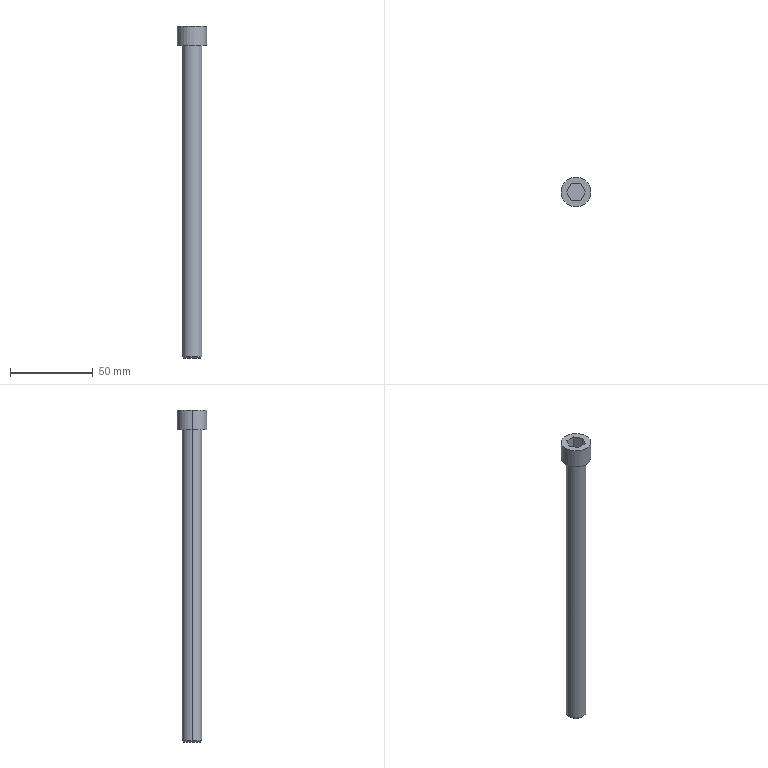Part | Creo | 1 solid | 16 faces | box 18 x 18 x 201 mm | volume 23734 mm3 | plane 10 | cylinder 4 | cone 2 | commonest cylinder face diameters 12 x2 18 x2
STEP:
#1=CARTESIAN_POINT('',(0.,0.,0.));
#2=DIRECTION('',(0.,0.,1.));
#3=DIRECTION('',(1.,0.,0.));
#4=AXIS2_PLACEMENT_3D('',#1,#2,#3);
#5=CARTESIAN_POINT('',(190.927,265.543,96.956));
#6=VERTEX_POINT('',#5);
#7=CARTESIAN_POINT('',(202.927,265.543,96.956));
#8=VERTEX_POINT('',#7);
#9=CARTESIAN_POINT('',(196.927,265.543,96.956));
#10=DIRECTION('',(0.,0.,-1.));
#11=DIRECTION('',(-1.,0.,0.));
#12=AXIS2_PLACEMENT_3D('',#9,#10,#11);
#13=CIRCLE('',#12,6.);
#14=EDGE_CURVE('',#6,#8,#13,.T.);
#15=ORIENTED_EDGE('',*,*,#14,.T.);
#16=CARTESIAN_POINT('',(202.927,265.543,285.245));
#17=VERTEX_POINT('',#16);
#18=CARTESIAN_POINT('',(202.927,265.543,285.245));
#19=DIRECTION('',(0.,0.,-1.));
#20=VECTOR('',#19,188.29);
#21=LINE('',#18,#20);
#22=EDGE_CURVE('',#17,#8,#21,.T.);
#23=ORIENTED_EDGE('',*,*,#22,.F.);
#24=CARTESIAN_POINT('',(190.927,265.543,285.245));
#25=VERTEX_POINT('',#24);
#26=CARTESIAN_POINT('',(196.927,265.543,285.245));
#27=DIRECTION('',(0.,0.,1.));
#28=DIRECTION('',(1.,0.,0.));
#29=AXIS2_PLACEMENT_3D('',#26,#27,#28);
#30=CIRCLE('',#29,6.);
#31=EDGE_CURVE('',#17,#25,#30,.T.);
#32=ORIENTED_EDGE('',*,*,#31,.T.);
#33=CARTESIAN_POINT('',(190.927,265.543,285.245));
#34=DIRECTION('',(0.,0.,-1.));
#35=VECTOR('',#34,188.29);
#36=LINE('',#33,#35);
#37=EDGE_CURVE('',#25,#6,#36,.T.);
#38=ORIENTED_EDGE('',*,*,#37,.T.);
#39=EDGE_LOOP('',(#15,#23,#32,#38));
#40=FACE_OUTER_BOUND('',#39,.F.);
#41=CARTESIAN_POINT('',(196.927,265.543,285.245));
#42=DIRECTION('',(0.,0.,-1.));
#43=DIRECTION('',(-1.,0.,0.));
#44=AXIS2_PLACEMENT_3D('',#41,#42,#43);
#45=CYLINDRICAL_SURFACE('',#44,6.);
#46=ADVANCED_FACE('',(#40),#45,.T.);
#47=CARTESIAN_POINT('',(191.637,265.543,96.245));
#48=VERTEX_POINT('',#47);
#49=CARTESIAN_POINT('',(202.216,265.543,96.245));
#50=VERTEX_POINT('',#49);
#51=CARTESIAN_POINT('',(196.927,265.543,96.245));
#52=DIRECTION('',(0.,0.,-1.));
#53=DIRECTION('',(-1.,0.,0.));
#54=AXIS2_PLACEMENT_3D('',#51,#52,#53);
#55=CIRCLE('',#54,5.29);
#56=EDGE_CURVE('',#48,#50,#55,.T.);
#57=ORIENTED_EDGE('',*,*,#56,.T.);
#58=CARTESIAN_POINT('',(202.216,265.543,96.245));
#59=DIRECTION('',(0.7071,0.,0.7071));
#60=VECTOR('',#59,1.005);
#61=LINE('',#58,#60);
#62=EDGE_CURVE('',#50,#8,#61,.T.);
#63=ORIENTED_EDGE('',*,*,#62,.T.);
#64=ORIENTED_EDGE('',*,*,#14,.F.);
#65=CARTESIAN_POINT('',(191.637,265.543,96.245));
#66=DIRECTION('',(-0.7071,0.,0.7071));
#67=VECTOR('',#66,1.005);
#68=LINE('',#65,#67);
#69=EDGE_CURVE('',#48,#6,#68,.T.);
#70=ORIENTED_EDGE('',*,*,#69,.F.);
#71=EDGE_LOOP('',(#57,#63,#64,#70));
#72=FACE_OUTER_BOUND('',#71,.F.);
#73=CARTESIAN_POINT('',(196.927,265.543,96.601));
#74=DIRECTION('',(0.,0.,1.));
#75=DIRECTION('',(1.,0.,0.));
#76=AXIS2_PLACEMENT_3D('',#73,#74,#75);
#77=CONICAL_SURFACE('',#76,5.645,45.);
#78=ADVANCED_FACE('',(#72),#77,.T.);
#79=CARTESIAN_POINT('',(196.927,265.543,96.245));
#80=DIRECTION('',(0.,0.,-1.));
#81=DIRECTION('',(1.,0.,0.));
#82=AXIS2_PLACEMENT_3D('',#79,#80,#81);
#83=CIRCLE('',#82,5.29);
#84=EDGE_CURVE('',#50,#48,#83,.T.);
#85=ORIENTED_EDGE('',*,*,#84,.F.);
#86=ORIENTED_EDGE('',*,*,#56,.F.);
#87=EDGE_LOOP('',(#85,#86));
#88=FACE_OUTER_BOUND('',#87,.F.);
#89=CARTESIAN_POINT('',(196.927,265.543,96.245));
#90=DIRECTION('',(0.,0.,1.));
#91=DIRECTION('',(1.,0.,0.));
#92=AXIS2_PLACEMENT_3D('',#89,#90,#91);
#93=PLANE('',#92);
#94=ADVANCED_FACE('',(#88),#93,.F.);
#95=ORIENTED_EDGE('',*,*,#84,.T.);
#96=ORIENTED_EDGE('',*,*,#69,.T.);
#97=CARTESIAN_POINT('',(196.927,265.543,96.956));
#98=DIRECTION('',(0.,0.,-1.));
#99=DIRECTION('',(1.,0.,0.));
#100=AXIS2_PLACEMENT_3D('',#97,#98,#99);
#101=CIRCLE('',#100,6.);
#102=EDGE_CURVE('',#8,#6,#101,.T.);
#103=ORIENTED_EDGE('',*,*,#102,.F.);
#104=ORIENTED_EDGE('',*,*,#62,.F.);
#105=EDGE_LOOP('',(#95,#96,#103,#104));
#106=FACE_OUTER_BOUND('',#105,.F.);
#107=CARTESIAN_POINT('',(196.927,265.543,96.601));
#108=DIRECTION('',(0.,0.,1.));
#109=DIRECTION('',(1.,0.,0.));
#110=AXIS2_PLACEMENT_3D('',#107,#108,#109);
#111=CONICAL_SURFACE('',#110,5.645,45.);
#112=ADVANCED_FACE('',(#106),#111,.T.);
#113=ORIENTED_EDGE('',*,*,#102,.T.);
#114=ORIENTED_EDGE('',*,*,#37,.F.);
#115=CARTESIAN_POINT('',(196.927,265.543,285.245));
#116=DIRECTION('',(0.,0.,1.));
#117=DIRECTION('',(-1.,0.,0.));
#118=AXIS2_PLACEMENT_3D('',#115,#116,#117);
#119=CIRCLE('',#118,6.);
#120=EDGE_CURVE('',#25,#17,#119,.T.);
#121=ORIENTED_EDGE('',*,*,#120,.T.);
#122=ORIENTED_EDGE('',*,*,#22,.T.);
#123=EDGE_LOOP('',(#113,#114,#121,#122));
#124=FACE_OUTER_BOUND('',#123,.F.);
#125=CARTESIAN_POINT('',(196.927,265.543,285.245));
#126=DIRECTION('',(0.,0.,-1.));
#127=DIRECTION('',(-1.,0.,0.));
#128=AXIS2_PLACEMENT_3D('',#125,#126,#127);
#129=CYLINDRICAL_SURFACE('',#128,6.);
#130=ADVANCED_FACE('',(#124),#129,.T.);
#131=CARTESIAN_POINT('',(205.927,265.543,285.245));
#132=VERTEX_POINT('',#131);
#133=CARTESIAN_POINT('',(187.927,265.543,285.245));
#134=VERTEX_POINT('',#133);
#135=CARTESIAN_POINT('',(196.927,265.543,285.245));
#136=DIRECTION('',(0.,0.,-1.));
#137=DIRECTION('',(1.,0.,0.));
#138=AXIS2_PLACEMENT_3D('',#135,#136,#137);
#139=CIRCLE('',#138,9.);
#140=EDGE_CURVE('',#132,#134,#139,.T.);
#141=ORIENTED_EDGE('',*,*,#140,.F.);
#142=CARTESIAN_POINT('',(196.927,265.543,285.245));
#143=DIRECTION('',(0.,0.,-1.));
#144=DIRECTION('',(-1.,0.,0.));
#145=AXIS2_PLACEMENT_3D('',#142,#143,#144);
#146=CIRCLE('',#145,9.);
#147=EDGE_CURVE('',#134,#132,#146,.T.);
#148=ORIENTED_EDGE('',*,*,#147,.F.);
#149=EDGE_LOOP('',(#141,#148));
#150=FACE_OUTER_BOUND('',#149,.F.);
#151=ORIENTED_EDGE('',*,*,#31,.F.);
#152=ORIENTED_EDGE('',*,*,#120,.F.);
#153=EDGE_LOOP('',(#151,#152));
#154=FACE_BOUND('',#153,.F.);
#155=CARTESIAN_POINT('',(196.927,265.543,285.245));
#156=DIRECTION('',(0.,0.,-1.));
#157=DIRECTION('',(-1.,0.,0.));
#158=AXIS2_PLACEMENT_3D('',#155,#156,#157);
#159=PLANE('',#158);
#160=ADVANCED_FACE('',(#150,#154),#159,.T.);
#161=CARTESIAN_POINT('',(187.927,265.543,297.245));
#162=VERTEX_POINT('',#161);
#163=CARTESIAN_POINT('',(205.927,265.543,297.245));
#164=VERTEX_POINT('',#163);
#165=CARTESIAN_POINT('',(196.927,265.543,297.245));
#166=DIRECTION('',(0.,0.,1.));
#167=DIRECTION('',(-1.,0.,0.));
#168=AXIS2_PLACEMENT_3D('',#165,#166,#167);
#169=CIRCLE('',#168,9.);
#170=EDGE_CURVE('',#162,#164,#169,.T.);
#171=ORIENTED_EDGE('',*,*,#170,.T.);
#172=CARTESIAN_POINT('',(205.927,265.543,285.245));
#173=DIRECTION('',(0.,0.,1.));
#174=VECTOR('',#173,12.);
#175=LINE('',#172,#174);
#176=EDGE_CURVE('',#132,#164,#175,.T.);
#177=ORIENTED_EDGE('',*,*,#176,.F.);
#178=ORIENTED_EDGE('',*,*,#140,.T.);
#179=CARTESIAN_POINT('',(187.927,265.543,285.245));
#180=DIRECTION('',(0.,0.,1.));
#181=VECTOR('',#180,12.);
#182=LINE('',#179,#181);
#183=EDGE_CURVE('',#134,#162,#182,.T.);
#184=ORIENTED_EDGE('',*,*,#183,.T.);
#185=EDGE_LOOP('',(#171,#177,#178,#184));
#186=FACE_OUTER_BOUND('',#185,.F.);
#187=CARTESIAN_POINT('',(196.927,265.543,285.245));
#188=DIRECTION('',(0.,0.,1.));
#189=DIRECTION('',(1.,0.,0.));
#190=AXIS2_PLACEMENT_3D('',#187,#188,#189);
#191=CYLINDRICAL_SURFACE('',#190,9.);
#192=ADVANCED_FACE('',(#186),#191,.T.);
#193=CARTESIAN_POINT('',(196.927,265.543,297.245));
#194=DIRECTION('',(0.,0.,1.));
#195=DIRECTION('',(1.,0.,0.));
#196=AXIS2_PLACEMENT_3D('',#193,#194,#195);
#197=CIRCLE('',#196,9.);
#198=EDGE_CURVE('',#164,#162,#197,.T.);
#199=ORIENTED_EDGE('',*,*,#198,.F.);
#200=ORIENTED_EDGE('',*,*,#170,.F.);
#201=EDGE_LOOP('',(#199,#200));
#202=FACE_OUTER_BOUND('',#201,.F.);
#203=CARTESIAN_POINT('',(199.813,260.543,297.245));
#204=VERTEX_POINT('',#203);
#205=CARTESIAN_POINT('',(194.04,260.543,297.245));
#206=VERTEX_POINT('',#205);
#207=CARTESIAN_POINT('',(199.813,260.543,297.245));
#208=DIRECTION('',(-1.,0.,0.));
#209=VECTOR('',#208,5.774);
#210=LINE('',#207,#209);
#211=EDGE_CURVE('',#204,#206,#210,.T.);
#212=ORIENTED_EDGE('',*,*,#211,.F.);
#213=CARTESIAN_POINT('',(202.7,265.543,297.245));
#214=VERTEX_POINT('',#213);
#215=CARTESIAN_POINT('',(202.7,265.543,297.245));
#216=DIRECTION('',(-0.5,-0.866,0.));
#217=VECTOR('',#216,5.774);
#218=LINE('',#215,#217);
#219=EDGE_CURVE('',#214,#204,#218,.T.);
#220=ORIENTED_EDGE('',*,*,#219,.F.);
#221=CARTESIAN_POINT('',(199.813,270.543,297.245));
#222=VERTEX_POINT('',#221);
#223=CARTESIAN_POINT('',(199.813,270.543,297.245));
#224=DIRECTION('',(0.5,-0.866,0.));
#225=VECTOR('',#224,5.774);
#226=LINE('',#223,#225);
#227=EDGE_CURVE('',#222,#214,#226,.T.);
#228=ORIENTED_EDGE('',*,*,#227,.F.);
#229=CARTESIAN_POINT('',(194.04,270.543,297.245));
#230=VERTEX_POINT('',#229);
#231=CARTESIAN_POINT('',(194.04,270.543,297.245));
#232=DIRECTION('',(1.,0.,0.));
#233=VECTOR('',#232,5.774);
#234=LINE('',#231,#233);
#235=EDGE_CURVE('',#230,#222,#234,.T.);
#236=ORIENTED_EDGE('',*,*,#235,.F.);
#237=CARTESIAN_POINT('',(191.153,265.543,297.245));
#238=VERTEX_POINT('',#237);
#239=CARTESIAN_POINT('',(191.153,265.543,297.245));
#240=DIRECTION('',(0.5,0.866,0.));
#241=VECTOR('',#240,5.774);
#242=LINE('',#239,#241);
#243=EDGE_CURVE('',#238,#230,#242,.T.);
#244=ORIENTED_EDGE('',*,*,#243,.F.);
#245=CARTESIAN_POINT('',(194.04,260.543,297.245));
#246=DIRECTION('',(-0.5,0.866,0.));
#247=VECTOR('',#246,5.774);
#248=LINE('',#245,#247);
#249=EDGE_CURVE('',#206,#238,#248,.T.);
#250=ORIENTED_EDGE('',*,*,#249,.F.);
#251=EDGE_LOOP('',(#212,#220,#228,#236,#244,#250));
#252=FACE_BOUND('',#251,.F.);
#253=CARTESIAN_POINT('',(196.927,265.543,297.245));
#254=DIRECTION('',(0.,0.,1.));
#255=DIRECTION('',(1.,0.,0.));
#256=AXIS2_PLACEMENT_3D('',#253,#254,#255);
#257=PLANE('',#256);
#258=ADVANCED_FACE('',(#202,#252),#257,.T.);
#259=ORIENTED_EDGE('',*,*,#211,.T.);
#260=CARTESIAN_POINT('',(194.04,260.543,289.325));
#261=VERTEX_POINT('',#260);
#262=CARTESIAN_POINT('',(194.04,260.543,297.245));
#263=DIRECTION('',(0.,0.,-1.));
#264=VECTOR('',#263,7.92);
#265=LINE('',#262,#264);
#266=EDGE_CURVE('',#206,#261,#265,.T.);
#267=ORIENTED_EDGE('',*,*,#266,.T.);
#268=CARTESIAN_POINT('',(199.813,260.543,289.325));
#269=VERTEX_POINT('',#268);
#270=CARTESIAN_POINT('',(199.813,260.543,289.325));
#271=DIRECTION('',(-1.,0.,0.));
#272=VECTOR('',#271,5.774);
#273=LINE('',#270,#272);
#274=EDGE_CURVE('',#269,#261,#273,.T.);
#275=ORIENTED_EDGE('',*,*,#274,.F.);
#276=CARTESIAN_POINT('',(199.813,260.543,297.245));
#277=DIRECTION('',(0.,0.,-1.));
#278=VECTOR('',#277,7.92);
#279=LINE('',#276,#278);
#280=EDGE_CURVE('',#204,#269,#279,.T.);
#281=ORIENTED_EDGE('',*,*,#280,.F.);
#282=EDGE_LOOP('',(#259,#267,#275,#281));
#283=FACE_OUTER_BOUND('',#282,.F.);
#284=CARTESIAN_POINT('',(194.04,260.543,289.325));
#285=DIRECTION('',(0.,-1.,0.));
#286=DIRECTION('',(0.,0.,-1.));
#287=AXIS2_PLACEMENT_3D('',#284,#285,#286);
#288=PLANE('',#287);
#289=ADVANCED_FACE('',(#283),#288,.F.);
#290=ORIENTED_EDGE('',*,*,#249,.T.);
#291=CARTESIAN_POINT('',(191.153,265.543,289.325));
#292=VERTEX_POINT('',#291);
#293=CARTESIAN_POINT('',(191.153,265.543,297.245));
#294=DIRECTION('',(0.,0.,-1.));
#295=VECTOR('',#294,7.92);
#296=LINE('',#293,#295);
#297=EDGE_CURVE('',#238,#292,#296,.T.);
#298=ORIENTED_EDGE('',*,*,#297,.T.);
#299=CARTESIAN_POINT('',(191.153,265.543,289.325));
#300=DIRECTION('',(0.5,-0.866,0.));
#301=VECTOR('',#300,5.774);
#302=LINE('',#299,#301);
#303=EDGE_CURVE('',#292,#261,#302,.T.);
#304=ORIENTED_EDGE('',*,*,#303,.T.);
#305=ORIENTED_EDGE('',*,*,#266,.F.);
#306=EDGE_LOOP('',(#290,#298,#304,#305));
#307=FACE_OUTER_BOUND('',#306,.F.);
#308=CARTESIAN_POINT('',(191.153,265.543,289.325));
#309=DIRECTION('',(-0.866,-0.5,0.));
#310=DIRECTION('',(0.5,-0.866,0.));
#311=AXIS2_PLACEMENT_3D('',#308,#309,#310);
#312=PLANE('',#311);
#313=ADVANCED_FACE('',(#307),#312,.F.);
#314=ORIENTED_EDGE('',*,*,#243,.T.);
#315=CARTESIAN_POINT('',(194.04,270.543,289.325));
#316=VERTEX_POINT('',#315);
#317=CARTESIAN_POINT('',(194.04,270.543,297.245));
#318=DIRECTION('',(0.,0.,-1.));
#319=VECTOR('',#318,7.92);
#320=LINE('',#317,#319);
#321=EDGE_CURVE('',#230,#316,#320,.T.);
#322=ORIENTED_EDGE('',*,*,#321,.T.);
#323=CARTESIAN_POINT('',(194.04,270.543,289.325));
#324=DIRECTION('',(-0.5,-0.866,0.));
#325=VECTOR('',#324,5.774);
#326=LINE('',#323,#325);
#327=EDGE_CURVE('',#316,#292,#326,.T.);
#328=ORIENTED_EDGE('',*,*,#327,.T.);
#329=ORIENTED_EDGE('',*,*,#297,.F.);
#330=EDGE_LOOP('',(#314,#322,#328,#329));
#331=FACE_OUTER_BOUND('',#330,.F.);
#332=CARTESIAN_POINT('',(194.04,270.543,289.325));
#333=DIRECTION('',(-0.866,0.5,0.));
#334=DIRECTION('',(-0.5,-0.866,0.));
#335=AXIS2_PLACEMENT_3D('',#332,#333,#334);
#336=PLANE('',#335);
#337=ADVANCED_FACE('',(#331),#336,.F.);
#338=ORIENTED_EDGE('',*,*,#235,.T.);
#339=CARTESIAN_POINT('',(199.813,270.543,289.325));
#340=VERTEX_POINT('',#339);
#341=CARTESIAN_POINT('',(199.813,270.543,297.245));
#342=DIRECTION('',(0.,0.,-1.));
#343=VECTOR('',#342,7.92);
#344=LINE('',#341,#343);
#345=EDGE_CURVE('',#222,#340,#344,.T.);
#346=ORIENTED_EDGE('',*,*,#345,.T.);
#347=CARTESIAN_POINT('',(194.04,270.543,289.325));
#348=DIRECTION('',(1.,0.,0.));
#349=VECTOR('',#348,5.774);
#350=LINE('',#347,#349);
#351=EDGE_CURVE('',#316,#340,#350,.T.);
#352=ORIENTED_EDGE('',*,*,#351,.F.);
#353=ORIENTED_EDGE('',*,*,#321,.F.);
#354=EDGE_LOOP('',(#338,#346,#352,#353));
#355=FACE_OUTER_BOUND('',#354,.F.);
#356=CARTESIAN_POINT('',(199.813,270.543,289.325));
#357=DIRECTION('',(0.,1.,0.));
#358=DIRECTION('',(0.,0.,1.));
#359=AXIS2_PLACEMENT_3D('',#356,#357,#358);
#360=PLANE('',#359);
#361=ADVANCED_FACE('',(#355),#360,.F.);
#362=ORIENTED_EDGE('',*,*,#227,.T.);
#363=CARTESIAN_POINT('',(202.7,265.543,289.325));
#364=VERTEX_POINT('',#363);
#365=CARTESIAN_POINT('',(202.7,265.543,297.245));
#366=DIRECTION('',(0.,0.,-1.));
#367=VECTOR('',#366,7.92);
#368=LINE('',#365,#367);
#369=EDGE_CURVE('',#214,#364,#368,.T.);
#370=ORIENTED_EDGE('',*,*,#369,.T.);
#371=CARTESIAN_POINT('',(202.7,265.543,289.325));
#372=DIRECTION('',(-0.5,0.866,0.));
#373=VECTOR('',#372,5.774);
#374=LINE('',#371,#373);
#375=EDGE_CURVE('',#364,#340,#374,.T.);
#376=ORIENTED_EDGE('',*,*,#375,.T.);
#377=ORIENTED_EDGE('',*,*,#345,.F.);
#378=EDGE_LOOP('',(#362,#370,#376,#377));
#379=FACE_OUTER_BOUND('',#378,.F.);
#380=CARTESIAN_POINT('',(202.7,265.543,289.325));
#381=DIRECTION('',(0.866,0.5,0.));
#382=DIRECTION('',(-0.5,0.866,0.));
#383=AXIS2_PLACEMENT_3D('',#380,#381,#382);
#384=PLANE('',#383);
#385=ADVANCED_FACE('',(#379),#384,.F.);
#386=ORIENTED_EDGE('',*,*,#219,.T.);
#387=ORIENTED_EDGE('',*,*,#280,.T.);
#388=CARTESIAN_POINT('',(199.813,260.543,289.325));
#389=DIRECTION('',(0.5,0.866,0.));
#390=VECTOR('',#389,5.774);
#391=LINE('',#388,#390);
#392=EDGE_CURVE('',#269,#364,#391,.T.);
#393=ORIENTED_EDGE('',*,*,#392,.T.);
#394=ORIENTED_EDGE('',*,*,#369,.F.);
#395=EDGE_LOOP('',(#386,#387,#393,#394));
#396=FACE_OUTER_BOUND('',#395,.F.);
#397=CARTESIAN_POINT('',(199.813,260.543,289.325));
#398=DIRECTION('',(0.866,-0.5,0.));
#399=DIRECTION('',(0.5,0.866,0.));
#400=AXIS2_PLACEMENT_3D('',#397,#398,#399);
#401=PLANE('',#400);
#402=ADVANCED_FACE('',(#396),#401,.F.);
#403=ORIENTED_EDGE('',*,*,#274,.T.);
#404=ORIENTED_EDGE('',*,*,#303,.F.);
#405=ORIENTED_EDGE('',*,*,#327,.F.);
#406=ORIENTED_EDGE('',*,*,#351,.T.);
#407=ORIENTED_EDGE('',*,*,#375,.F.);
#408=ORIENTED_EDGE('',*,*,#392,.F.);
#409=EDGE_LOOP('',(#403,#404,#405,#406,#407,#408));
#410=FACE_OUTER_BOUND('',#409,.F.);
#411=CARTESIAN_POINT('',(199.813,260.543,289.325));
#412=DIRECTION('',(0.,0.,1.));
#413=DIRECTION('',(1.,0.,0.));
#414=AXIS2_PLACEMENT_3D('',#411,#412,#413);
#415=PLANE('',#414);
#416=ADVANCED_FACE('',(#410),#415,.T.);
#417=ORIENTED_EDGE('',*,*,#198,.T.);
#418=ORIENTED_EDGE('',*,*,#183,.F.);
#419=ORIENTED_EDGE('',*,*,#147,.T.);
#420=ORIENTED_EDGE('',*,*,#176,.T.);
#421=EDGE_LOOP('',(#417,#418,#419,#420));
#422=FACE_OUTER_BOUND('',#421,.F.);
#423=CARTESIAN_POINT('',(196.927,265.543,285.245));
#424=DIRECTION('',(0.,0.,1.));
#425=DIRECTION('',(1.,0.,0.));
#426=AXIS2_PLACEMENT_3D('',#423,#424,#425);
#427=CYLINDRICAL_SURFACE('',#426,9.);
#428=ADVANCED_FACE('',(#422),#427,.T.);
#429=CLOSED_SHELL('',(#46,#78,#94,#112,#130,#160,#192,#258,#289,#313,#337,#361,#385,#402,#416,#428));
#430=MANIFOLD_SOLID_BREP('',#429);
#431=(LENGTH_UNIT()NAMED_UNIT(*)SI_UNIT(.MILLI.,.METRE.));
#432=UNCERTAINTY_MEASURE_WITH_UNIT(LENGTH_MEASURE(0.02026),#431,'','');
#433=(NAMED_UNIT(*)PLANE_ANGLE_UNIT()SI_UNIT($,.RADIAN.));
#434=PLANE_ANGLE_MEASURE_WITH_UNIT(PLANE_ANGLE_MEASURE(0.01745),#433);
#435=(CONVERSION_BASED_UNIT('DEGREE',#434)NAMED_UNIT(*)PLANE_ANGLE_UNIT());
#436=(NAMED_UNIT(*)SI_UNIT($,.STERADIAN.)SOLID_ANGLE_UNIT());
#437=(GEOMETRIC_REPRESENTATION_CONTEXT(3)GLOBAL_UNCERTAINTY_ASSIGNED_CONTEXT((#432))GLOBAL_UNIT_ASSIGNED_CONTEXT((#431,#435,#436))REPRESENTATION_CONTEXT('',''));
#438=ADVANCED_BREP_SHAPE_REPRESENTATION('',(#4,#430),#437);